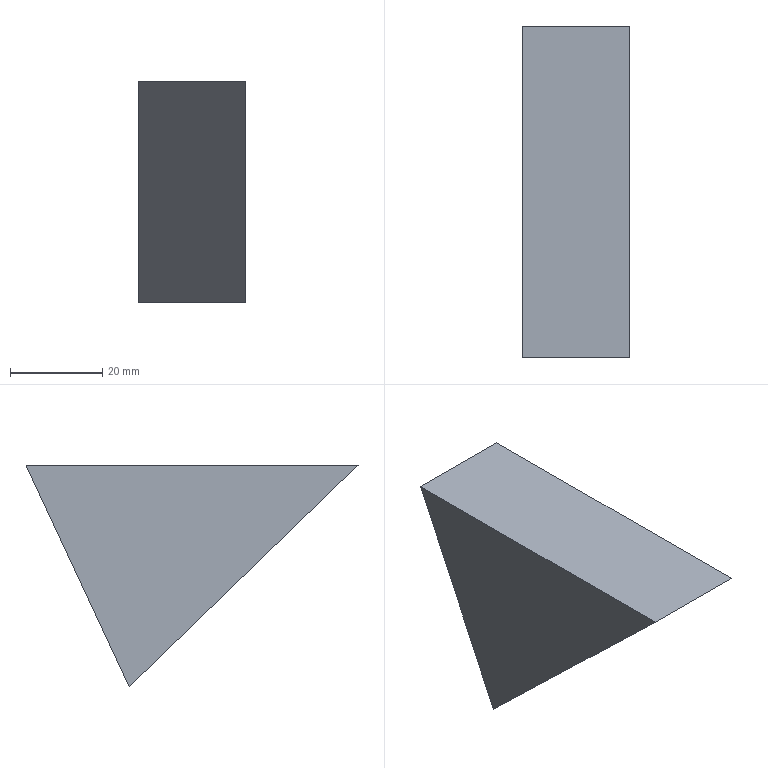Part | Creo | 1 solid | 5 faces | box 23.38 x 72.174 x 48.057 mm | volume 40546 mm3 | plane 5
STEP:
#1=CARTESIAN_POINT('',(0.,0.,0.));
#2=DIRECTION('',(0.,0.,1.));
#3=DIRECTION('',(1.,0.,0.));
#4=AXIS2_PLACEMENT_3D('',#1,#2,#3);
#5=CARTESIAN_POINT('',(41.118,145.852,-81.892));
#6=VERTEX_POINT('',#5);
#7=CARTESIAN_POINT('',(17.738,145.852,-81.892));
#8=VERTEX_POINT('',#7);
#9=CARTESIAN_POINT('',(41.118,145.852,-81.892));
#10=DIRECTION('',(-1.,0.000000014,-0.000000013));
#11=VECTOR('',#10,23.38);
#12=LINE('',#9,#11);
#13=EDGE_CURVE('',#6,#8,#12,.T.);
#14=ORIENTED_EDGE('',*,*,#13,.T.);
#15=CARTESIAN_POINT('',(17.738,96.087,-33.835));
#16=VERTEX_POINT('',#15);
#17=CARTESIAN_POINT('',(17.738,145.852,-81.892));
#18=DIRECTION('',(0.,-0.7193,0.6947));
#19=VECTOR('',#18,69.181);
#20=LINE('',#17,#19);
#21=EDGE_CURVE('',#8,#16,#20,.T.);
#22=ORIENTED_EDGE('',*,*,#21,.T.);
#23=CARTESIAN_POINT('',(41.118,96.087,-33.835));
#24=VERTEX_POINT('',#23);
#25=CARTESIAN_POINT('',(17.738,96.087,-33.835));
#26=DIRECTION('',(1.,-0.000000212,0.000000195));
#27=VECTOR('',#26,23.38);
#28=LINE('',#25,#27);
#29=EDGE_CURVE('',#16,#24,#28,.T.);
#30=ORIENTED_EDGE('',*,*,#29,.T.);
#31=CARTESIAN_POINT('',(41.118,96.087,-33.835));
#32=DIRECTION('',(-0.000000033,0.7193,-0.6947));
#33=VECTOR('',#32,69.181);
#34=LINE('',#31,#33);
#35=EDGE_CURVE('',#24,#6,#34,.T.);
#36=ORIENTED_EDGE('',*,*,#35,.T.);
#37=EDGE_LOOP('',(#14,#22,#30,#36));
#38=FACE_OUTER_BOUND('',#37,.F.);
#39=CARTESIAN_POINT('',(24.775,113.851,-50.989));
#40=DIRECTION('',(0.,0.6947,0.7193));
#41=DIRECTION('',(0.,-0.7193,0.6947));
#42=AXIS2_PLACEMENT_3D('',#39,#40,#41);
#43=PLANE('',#42);
#44=ADVANCED_FACE('',(#38),#43,.F.);
#45=CARTESIAN_POINT('',(41.118,168.261,-33.835));
#46=VERTEX_POINT('',#45);
#47=CARTESIAN_POINT('',(41.118,145.852,-81.892));
#48=DIRECTION('',(-0.000000019,0.4226,0.9063));
#49=VECTOR('',#48,53.025);
#50=LINE('',#47,#49);
#51=EDGE_CURVE('',#6,#46,#50,.T.);
#52=ORIENTED_EDGE('',*,*,#51,.T.);
#53=CARTESIAN_POINT('',(17.738,168.261,-33.835));
#54=VERTEX_POINT('',#53);
#55=CARTESIAN_POINT('',(17.738,168.261,-33.835));
#56=DIRECTION('',(1.,0.000000066,0.000000185));
#57=VECTOR('',#56,23.38);
#58=LINE('',#55,#57);
#59=EDGE_CURVE('',#54,#46,#58,.T.);
#60=ORIENTED_EDGE('',*,*,#59,.F.);
#61=CARTESIAN_POINT('',(17.738,168.261,-33.835));
#62=DIRECTION('',(0.,-0.4226,-0.9063));
#63=VECTOR('',#62,53.025);
#64=LINE('',#61,#63);
#65=EDGE_CURVE('',#54,#8,#64,.T.);
#66=ORIENTED_EDGE('',*,*,#65,.T.);
#67=ORIENTED_EDGE('',*,*,#13,.F.);
#68=EDGE_LOOP('',(#52,#60,#66,#67));
#69=FACE_OUTER_BOUND('',#68,.F.);
#70=CARTESIAN_POINT('',(17.598,145.717,-82.181));
#71=DIRECTION('',(0.000000018,0.9063,-0.4226));
#72=DIRECTION('',(0.,0.4226,0.9063));
#73=AXIS2_PLACEMENT_3D('',#70,#71,#72);
#74=PLANE('',#73);
#75=ADVANCED_FACE('',(#69),#74,.T.);
#76=ORIENTED_EDGE('',*,*,#35,.F.);
#77=CARTESIAN_POINT('',(41.118,96.087,-33.835));
#78=DIRECTION('',(-0.000000046,1.,-0.000000009));
#79=VECTOR('',#78,72.174);
#80=LINE('',#77,#79);
#81=EDGE_CURVE('',#24,#46,#80,.T.);
#82=ORIENTED_EDGE('',*,*,#81,.T.);
#83=ORIENTED_EDGE('',*,*,#51,.F.);
#84=EDGE_LOOP('',(#76,#82,#83));
#85=FACE_OUTER_BOUND('',#84,.F.);
#86=CARTESIAN_POINT('',(41.118,80.496,-15.998));
#87=DIRECTION('',(-1.,-0.000000046,0.));
#88=DIRECTION('',(0.000000046,-1.,0.));
#89=AXIS2_PLACEMENT_3D('',#86,#87,#88);
#90=PLANE('',#89);
#91=ADVANCED_FACE('',(#85),#90,.F.);
#92=ORIENTED_EDGE('',*,*,#81,.F.);
#93=ORIENTED_EDGE('',*,*,#29,.F.);
#94=CARTESIAN_POINT('',(17.738,96.087,-33.835));
#95=DIRECTION('',(0.,1.,-0.000000006));
#96=VECTOR('',#95,72.174);
#97=LINE('',#94,#96);
#98=EDGE_CURVE('',#16,#54,#97,.T.);
#99=ORIENTED_EDGE('',*,*,#98,.T.);
#100=ORIENTED_EDGE('',*,*,#59,.T.);
#101=EDGE_LOOP('',(#92,#93,#99,#100));
#102=FACE_OUTER_BOUND('',#101,.F.);
#103=CARTESIAN_POINT('',(-63.673,10000095.765,-33.835));
#104=DIRECTION('',(-0.000000175,0.,1.));
#105=DIRECTION('',(1.,0.,0.000000175));
#106=AXIS2_PLACEMENT_3D('',#103,#104,#105);
#107=PLANE('',#106);
#108=ADVANCED_FACE('',(#102),#107,.T.);
#109=ORIENTED_EDGE('',*,*,#65,.F.);
#110=ORIENTED_EDGE('',*,*,#98,.F.);
#111=ORIENTED_EDGE('',*,*,#21,.F.);
#112=EDGE_LOOP('',(#109,#110,#111));
#113=FACE_OUTER_BOUND('',#112,.F.);
#114=CARTESIAN_POINT('',(17.738,101.276,-38.757));
#115=DIRECTION('',(1.,0.,0.));
#116=DIRECTION('',(0.,0.,-1.));
#117=AXIS2_PLACEMENT_3D('',#114,#115,#116);
#118=PLANE('',#117);
#119=ADVANCED_FACE('',(#113),#118,.F.);
#120=CLOSED_SHELL('',(#44,#75,#91,#108,#119));
#121=MANIFOLD_SOLID_BREP('',#120);
#122=(LENGTH_UNIT()NAMED_UNIT(*)SI_UNIT(.MILLI.,.METRE.));
#123=UNCERTAINTY_MEASURE_WITH_UNIT(LENGTH_MEASURE(0.00898),#122,'','');
#124=(NAMED_UNIT(*)PLANE_ANGLE_UNIT()SI_UNIT($,.RADIAN.));
#125=PLANE_ANGLE_MEASURE_WITH_UNIT(PLANE_ANGLE_MEASURE(0.01745),#124);
#126=(CONVERSION_BASED_UNIT('DEGREE',#125)NAMED_UNIT(*)PLANE_ANGLE_UNIT());
#127=(NAMED_UNIT(*)SI_UNIT($,.STERADIAN.)SOLID_ANGLE_UNIT());
#128=(GEOMETRIC_REPRESENTATION_CONTEXT(3)GLOBAL_UNCERTAINTY_ASSIGNED_CONTEXT((#123))GLOBAL_UNIT_ASSIGNED_CONTEXT((#122,#126,#127))REPRESENTATION_CONTEXT('',''));
#129=ADVANCED_BREP_SHAPE_REPRESENTATION('',(#4,#121),#128);